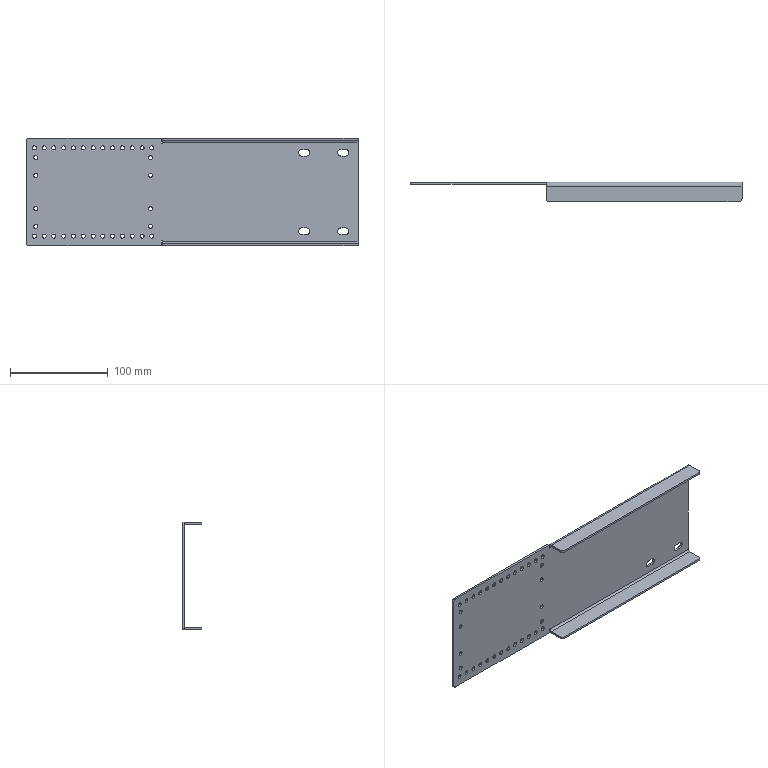Part | SolidWorks | features HoleWzd 3, EdgeFlange 1, Fillet 1, FlatPattern 1, ICE 1, SMBaseFlange 1, SheetMetal 1 | 1 solid | 120 faces | box 339 x 20 x 110 mm | volume 86427 mm3 | cylinder 86 | plane 34 | commonest cylinder face diameters 4.2 x68 6.6 x8 6 x6 4 x2 8 x2